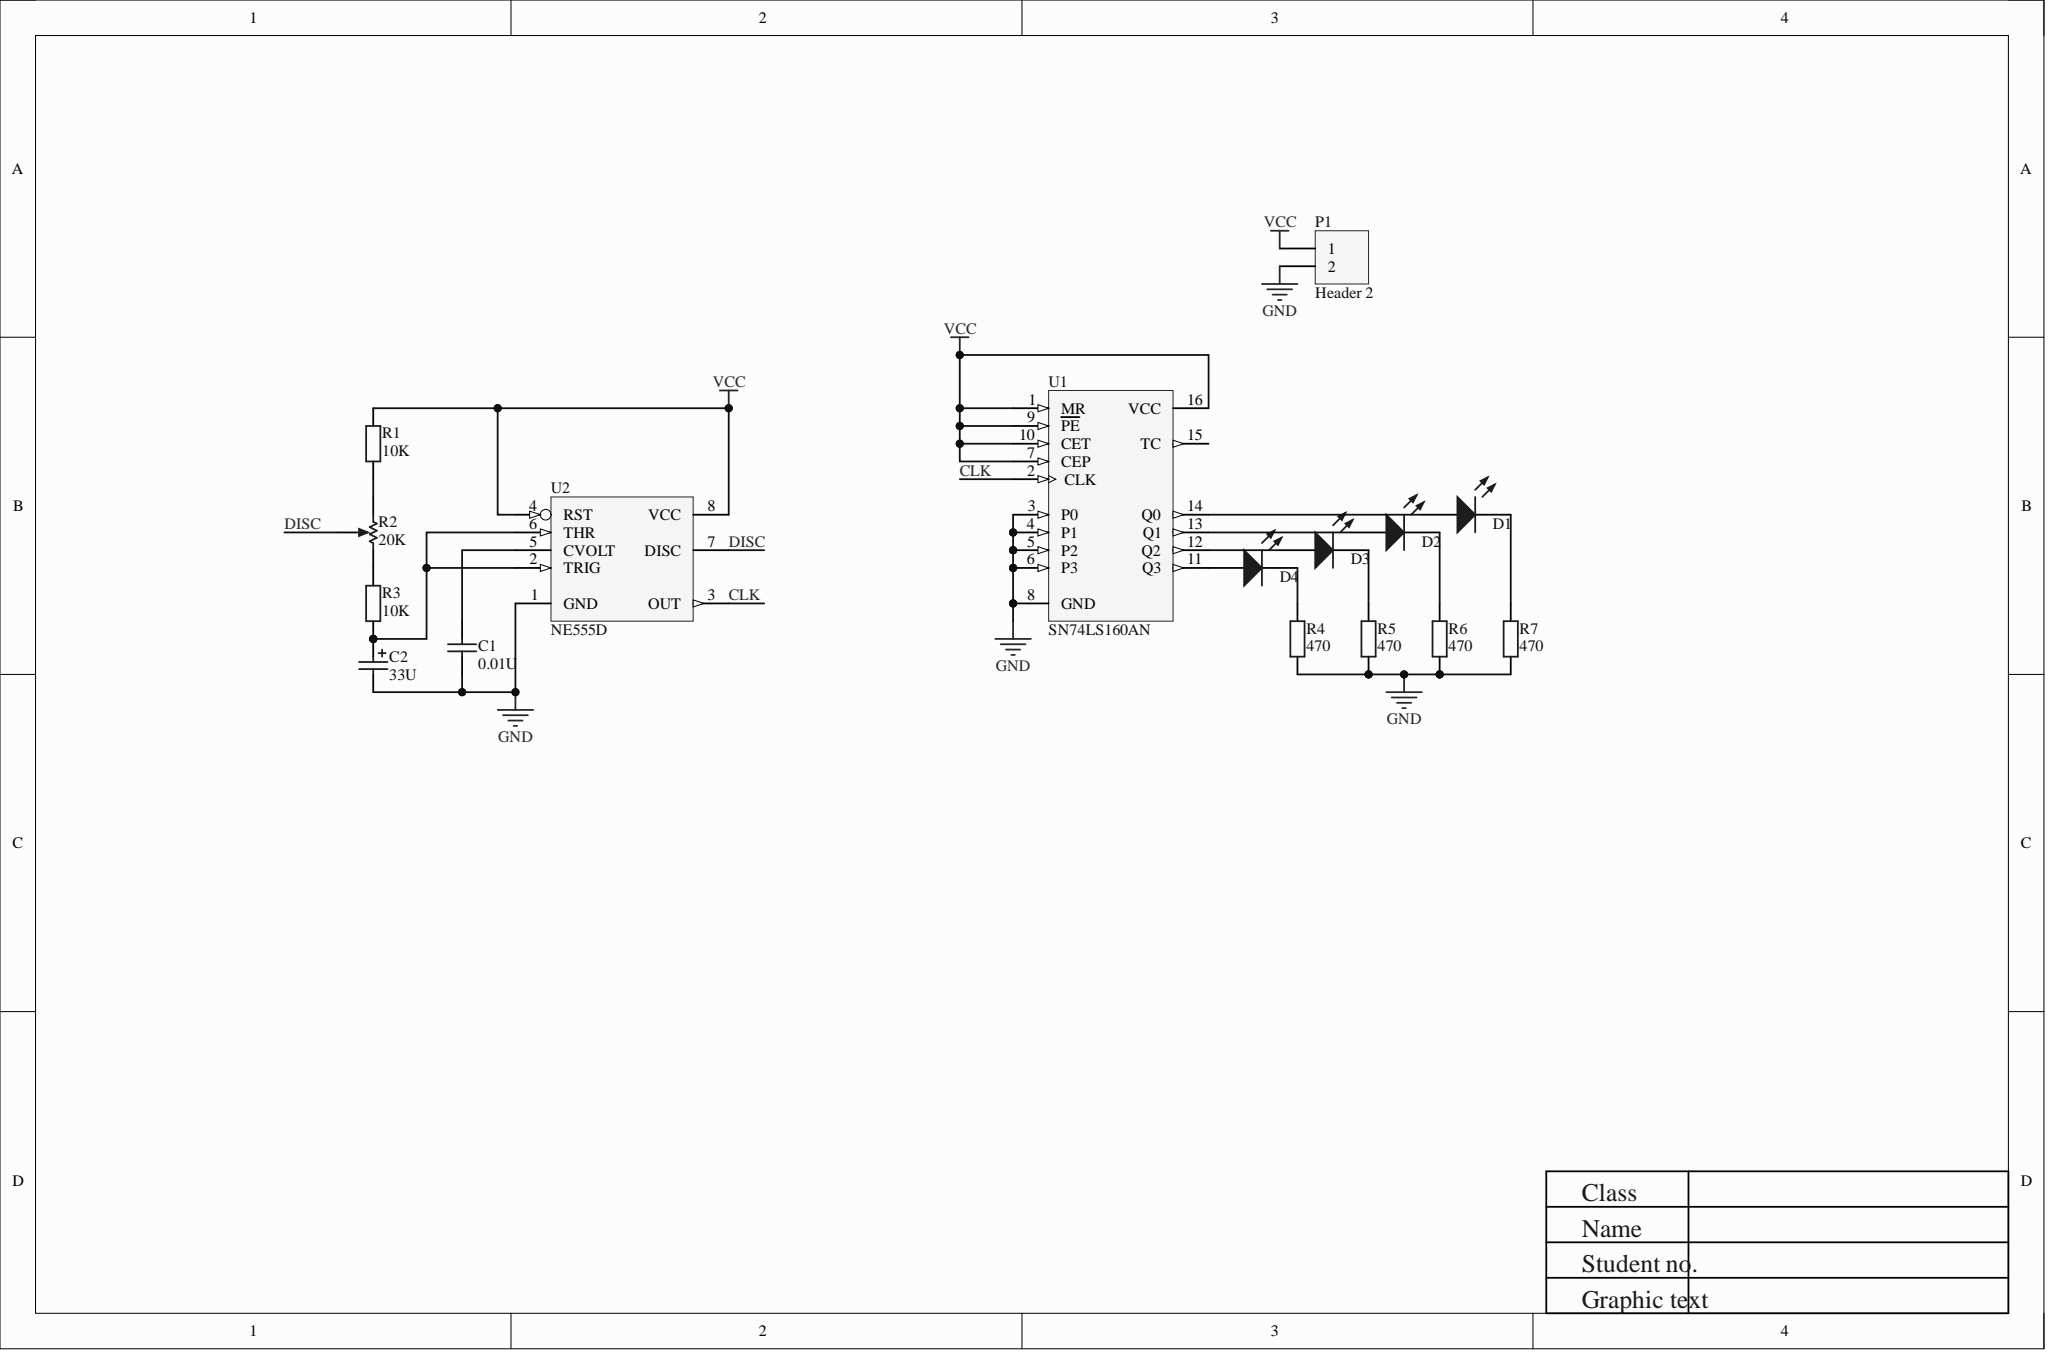Circuit board | Altium Designer | 16 parts | 16 nets
Bill of materials:
Comment,Description,Designator,Footprint,LibRef,Quantity
"0.01U","Capacitor","C1","RAD-0.3","Cap","1"
"33U","Polarized Capacitor (Axial)","C2","POLAR0.8","Cap Pol2","1"
"LED","Light-emitting diode","D1, D2, D3, D4","LED 5MM-W","LED","4"
"Header 2","Header, 2-Pin","P1","HDR1X2","Header 2","1"
"10K","Color-band resistor","R1, R3","RS 1/4W","R-S","2"
"20K","Potentiometer","R2","VR5","RPot","1"
"470","Color-band resistor","R4, R5, R6, R7","RS 1/4W","R-S","4"
"SN74LS160AN","BCD Decade Counter","U1","648-08","SN74LS160AN","1"
"NE555D","General-Purpose Single Bipolar Timer","U2","DIP8","NE555D","1"
Netlist (Protel format):
[
C1
RAD-0.3
0.01U



]
[
C2
POLAR0.8
33U



]
[
D1
LED 5MM-W
LED



]
[
D2
LED 5MM-W
LED



]
[
D3
LED 5MM-W
LED



]
[
D4
LED 5MM-W
LED



]
[
P1
HDR1X2
Header 2



]
[
R1
RS 1/4W
10K



]
[
R2
VR5
20K



]
[
R3
RS 1/4W
10K



]
[
R4
RS 1/4W
470



]
[
R5
RS 1/4W
470



]
[
R6
RS 1/4W
470



]
[
R7
RS 1/4W
470



]
[
U1
648-08
SN74LS160AN



]
[
U2
DIP8
NE555D



]
(
VCC
P1-1
R1-2
U1-1
U1-7
U1-9
U1-10
U1-16
U2-4
U2-8
)
(
NetR2_2
R2-2
R3-2
)
(
NetR1_1
R1-1
R2-1
)
(
NetD4_2
D4-2
R4-2
)
(
NetD4_1
D4-1
U1-11
)
(
NetD3_2
D3-2
R5-2
)
(
NetD3_1
D3-1
U1-12
)
(
NetD2_2
D2-2
R6-2
)
(
NetD2_1
D2-1
U1-13
)
(
NetD1_2
D1-2
R7-2
)
(
NetD1_1
D1-1
U1-14
)
(
NetC2_1
C2-1
R3-1
U2-2
U2-6
)
(
NetC1_2
C1-2
U2-5
)
(
GND
C1-1
C2-2
P1-2
R4-1
R5-1
R6-1
R7-1
U1-3
U1-4
U1-5
U1-6
U1-8
U2-1
)
(
DISC
R2-3
U2-7
)
(
CLK
U1-2
U2-3
)